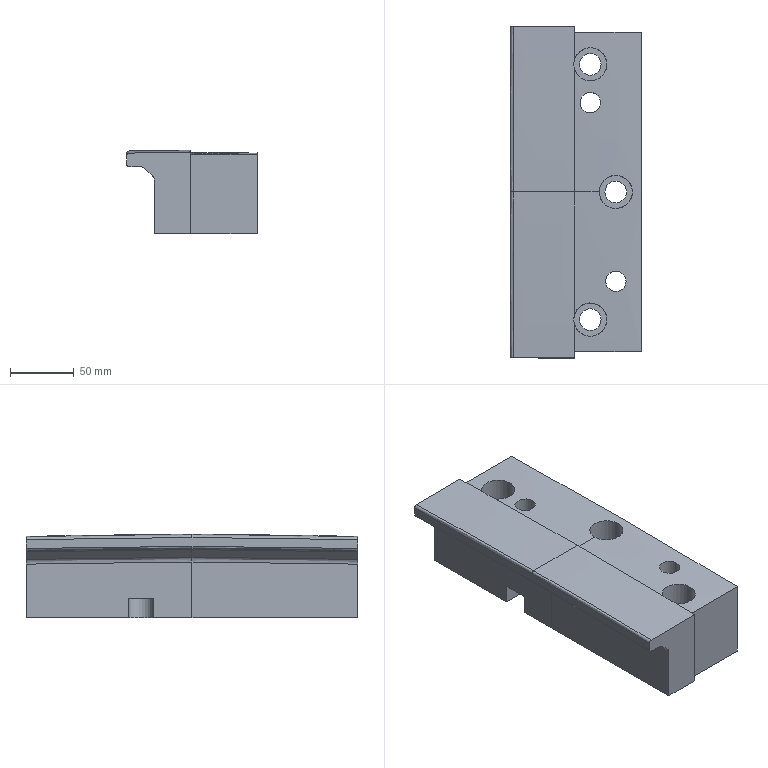Part | NX | features MAIN_BODY 2 | 1 solid | 43 faces | box 102.4 x 260 x 65.199 mm | volume 1240029 mm3 | spline 18 | plane 16 | cylinder 9 | commonest cylinder face diameters 17 x3 26 x3 16 x2 20 x1